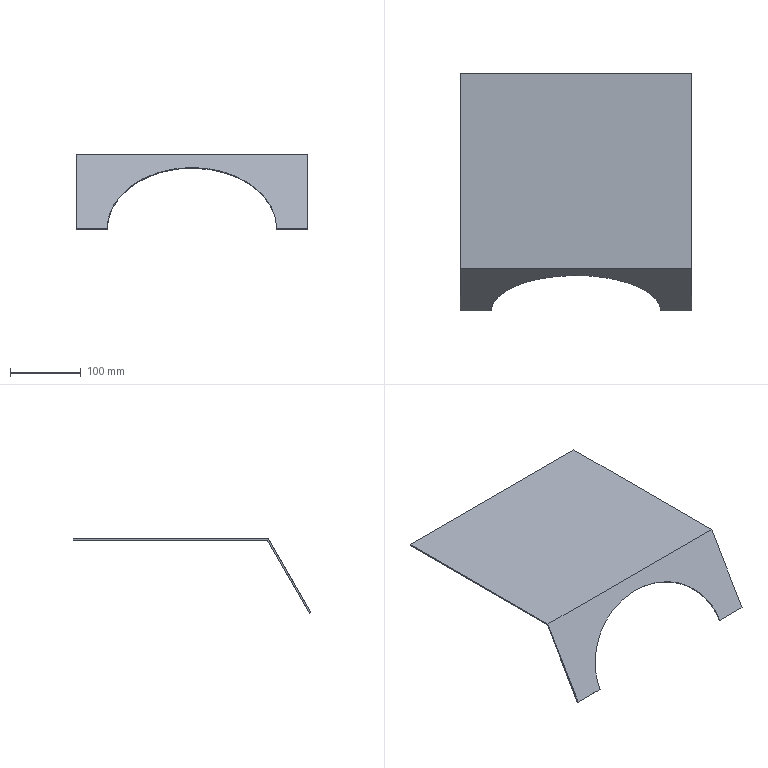Part | SolidWorks | features Attribute 3, ICE 2, Extrusion 1 | 1 solid | 10 faces | box 328 x 336.732 x 105.923 mm | volume 222158 mm3 | plane 9 | spline 1
STEP:
#1=CARTESIAN_POINT('',(-120.,-199.232,-102.923));
#2=VERTEX_POINT('',#1);
#3=CARTESIAN_POINT('',(-120.,-197.5,-103.923));
#4=VERTEX_POINT('',#3);
#5=CARTESIAN_POINT('',(-120.,-206.16,-98.923));
#6=DIRECTION('',(0.,0.866,-0.5));
#7=VECTOR('',#6,1000.);
#8=LINE('',#5,#7);
#9=EDGE_CURVE('',#2,#4,#8,.T.);
#10=ORIENTED_EDGE('',*,*,#9,.F.);
#11=CARTESIAN_POINT('',(-164.,-199.232,-102.923));
#12=VERTEX_POINT('',#11);
#13=CARTESIAN_POINT('',(286.599,-199.232,-102.923));
#14=DIRECTION('',(-1.,0.,0.));
#15=VECTOR('',#14,1000.);
#16=LINE('',#13,#15);
#17=EDGE_CURVE('',#2,#12,#16,.T.);
#18=ORIENTED_EDGE('',*,*,#17,.T.);
#19=CARTESIAN_POINT('',(-164.,-197.5,-103.923));
#20=VERTEX_POINT('',#19);
#21=CARTESIAN_POINT('',(-164.,-197.5,-103.923));
#22=DIRECTION('',(0.,-0.866,0.5));
#23=VECTOR('',#22,1000.);
#24=LINE('',#21,#23);
#25=EDGE_CURVE('',#20,#12,#24,.T.);
#26=ORIENTED_EDGE('',*,*,#25,.F.);
#27=CARTESIAN_POINT('',(286.599,-197.5,-103.923));
#28=DIRECTION('',(-1.,0.,0.));
#29=VECTOR('',#28,1000.);
#30=LINE('',#27,#29);
#31=EDGE_CURVE('',#4,#20,#30,.T.);
#32=ORIENTED_EDGE('',*,*,#31,.F.);
#33=EDGE_LOOP('',(#10,#18,#26,#32));
#34=FACE_OUTER_BOUND('',#33,.T.);
#35=CARTESIAN_POINT('',(286.599,-197.5,-103.923));
#36=DIRECTION('',(0.,-0.5,-0.866));
#37=DIRECTION('',(0.,0.866,-0.5));
#38=AXIS2_PLACEMENT_3D('',#35,#36,#37);
#39=PLANE('',#38);
#40=ADVANCED_FACE('',(#34),#39,.T.);
#41=CARTESIAN_POINT('',(164.,-137.5,0.));
#42=VERTEX_POINT('',#41);
#43=CARTESIAN_POINT('',(164.,137.5,0.));
#44=VERTEX_POINT('',#43);
#45=CARTESIAN_POINT('',(164.,137.5,0.));
#46=DIRECTION('',(0.,1.,0.));
#47=VECTOR('',#46,1000.);
#48=LINE('',#45,#47);
#49=EDGE_CURVE('',#42,#44,#48,.T.);
#50=ORIENTED_EDGE('',*,*,#49,.T.);
#51=CARTESIAN_POINT('',(164.,137.5,2.));
#52=VERTEX_POINT('',#51);
#53=CARTESIAN_POINT('',(164.,137.5,2.));
#54=DIRECTION('',(0.,0.,-1.));
#55=VECTOR('',#54,1000.);
#56=LINE('',#53,#55);
#57=EDGE_CURVE('',#52,#44,#56,.T.);
#58=ORIENTED_EDGE('',*,*,#57,.F.);
#59=CARTESIAN_POINT('',(164.,-138.655,2.));
#60=VERTEX_POINT('',#59);
#61=CARTESIAN_POINT('',(164.,137.5,2.));
#62=DIRECTION('',(0.,1.,0.));
#63=VECTOR('',#62,1000.);
#64=LINE('',#61,#63);
#65=EDGE_CURVE('',#60,#52,#64,.T.);
#66=ORIENTED_EDGE('',*,*,#65,.F.);
#67=CARTESIAN_POINT('',(164.,-199.232,-102.923));
#68=VERTEX_POINT('',#67);
#69=CARTESIAN_POINT('',(164.,-139.232,1.));
#70=DIRECTION('',(0.,-0.5,-0.866));
#71=VECTOR('',#70,1000.);
#72=LINE('',#69,#71);
#73=EDGE_CURVE('',#60,#68,#72,.T.);
#74=ORIENTED_EDGE('',*,*,#73,.T.);
#75=CARTESIAN_POINT('',(164.,-197.5,-103.923));
#76=VERTEX_POINT('',#75);
#77=CARTESIAN_POINT('',(164.,-197.5,-103.923));
#78=DIRECTION('',(0.,0.866,-0.5));
#79=VECTOR('',#78,1000.);
#80=LINE('',#77,#79);
#81=EDGE_CURVE('',#68,#76,#80,.T.);
#82=ORIENTED_EDGE('',*,*,#81,.T.);
#83=CARTESIAN_POINT('',(164.,-137.5,0.));
#84=DIRECTION('',(0.,0.5,0.866));
#85=VECTOR('',#84,1000.);
#86=LINE('',#83,#85);
#87=EDGE_CURVE('',#76,#42,#86,.T.);
#88=ORIENTED_EDGE('',*,*,#87,.T.);
#89=EDGE_LOOP('',(#50,#58,#66,#74,#82,#88));
#90=FACE_OUTER_BOUND('',#89,.T.);
#91=CARTESIAN_POINT('',(164.,137.5,2.));
#92=DIRECTION('',(-1.,0.,0.));
#93=DIRECTION('',(0.,-1.,0.));
#94=AXIS2_PLACEMENT_3D('',#91,#92,#93);
#95=PLANE('',#94);
#96=ADVANCED_FACE('',(#90),#95,.F.);
#97=CARTESIAN_POINT('',(-164.,137.5,0.));
#98=VERTEX_POINT('',#97);
#99=CARTESIAN_POINT('',(-164.,137.5,0.));
#100=DIRECTION('',(-1.,0.,0.));
#101=VECTOR('',#100,1000.);
#102=LINE('',#99,#101);
#103=EDGE_CURVE('',#44,#98,#102,.T.);
#104=ORIENTED_EDGE('',*,*,#103,.T.);
#105=CARTESIAN_POINT('',(-164.,137.5,2.));
#106=VERTEX_POINT('',#105);
#107=CARTESIAN_POINT('',(-164.,137.5,2.));
#108=DIRECTION('',(0.,0.,-1.));
#109=VECTOR('',#108,1000.);
#110=LINE('',#107,#109);
#111=EDGE_CURVE('',#106,#98,#110,.T.);
#112=ORIENTED_EDGE('',*,*,#111,.F.);
#113=CARTESIAN_POINT('',(-164.,137.5,2.));
#114=DIRECTION('',(-1.,0.,0.));
#115=VECTOR('',#114,1000.);
#116=LINE('',#113,#115);
#117=EDGE_CURVE('',#52,#106,#116,.T.);
#118=ORIENTED_EDGE('',*,*,#117,.F.);
#119=ORIENTED_EDGE('',*,*,#57,.T.);
#120=EDGE_LOOP('',(#104,#112,#118,#119));
#121=FACE_OUTER_BOUND('',#120,.T.);
#122=CARTESIAN_POINT('',(-164.,137.5,2.));
#123=DIRECTION('',(0.,-1.,0.));
#124=DIRECTION('',(0.,0.,-1.));
#125=AXIS2_PLACEMENT_3D('',#122,#123,#124);
#126=PLANE('',#125);
#127=ADVANCED_FACE('',(#121),#126,.F.);
#128=CARTESIAN_POINT('',(-164.,-137.5,0.));
#129=VERTEX_POINT('',#128);
#130=CARTESIAN_POINT('',(-164.,137.5,0.));
#131=DIRECTION('',(0.,-1.,0.));
#132=VECTOR('',#131,1000.);
#133=LINE('',#130,#132);
#134=EDGE_CURVE('',#98,#129,#133,.T.);
#135=ORIENTED_EDGE('',*,*,#134,.T.);
#136=CARTESIAN_POINT('',(-164.,-137.5,0.));
#137=DIRECTION('',(0.,-0.5,-0.866));
#138=VECTOR('',#137,1000.);
#139=LINE('',#136,#138);
#140=EDGE_CURVE('',#129,#20,#139,.T.);
#141=ORIENTED_EDGE('',*,*,#140,.T.);
#142=ORIENTED_EDGE('',*,*,#25,.T.);
#143=CARTESIAN_POINT('',(-164.,-138.655,2.));
#144=VERTEX_POINT('',#143);
#145=CARTESIAN_POINT('',(-164.,-139.232,1.));
#146=DIRECTION('',(0.,0.5,0.866));
#147=VECTOR('',#146,1000.);
#148=LINE('',#145,#147);
#149=EDGE_CURVE('',#12,#144,#148,.T.);
#150=ORIENTED_EDGE('',*,*,#149,.T.);
#151=CARTESIAN_POINT('',(-164.,137.5,2.));
#152=DIRECTION('',(0.,-1.,0.));
#153=VECTOR('',#152,1000.);
#154=LINE('',#151,#153);
#155=EDGE_CURVE('',#106,#144,#154,.T.);
#156=ORIENTED_EDGE('',*,*,#155,.F.);
#157=ORIENTED_EDGE('',*,*,#111,.T.);
#158=EDGE_LOOP('',(#135,#141,#142,#150,#156,#157));
#159=FACE_OUTER_BOUND('',#158,.T.);
#160=CARTESIAN_POINT('',(-164.,137.5,2.));
#161=DIRECTION('',(1.,0.,0.));
#162=DIRECTION('',(0.,1.,0.));
#163=AXIS2_PLACEMENT_3D('',#160,#161,#162);
#164=PLANE('',#163);
#165=ADVANCED_FACE('',(#159),#164,.F.);
#166=ORIENTED_EDGE('',*,*,#65,.T.);
#167=ORIENTED_EDGE('',*,*,#117,.T.);
#168=ORIENTED_EDGE('',*,*,#155,.T.);
#169=CARTESIAN_POINT('',(286.599,-138.655,2.));
#170=DIRECTION('',(-1.,0.,0.));
#171=VECTOR('',#170,1000.);
#172=LINE('',#169,#171);
#173=EDGE_CURVE('',#60,#144,#172,.T.);
#174=ORIENTED_EDGE('',*,*,#173,.F.);
#175=EDGE_LOOP('',(#166,#167,#168,#174));
#176=FACE_OUTER_BOUND('',#175,.T.);
#177=CARTESIAN_POINT('',(0.,0.,2.));
#178=DIRECTION('',(0.,0.,1.));
#179=DIRECTION('',(1.,0.,0.));
#180=AXIS2_PLACEMENT_3D('',#177,#178,#179);
#181=PLANE('',#180);
#182=ADVANCED_FACE('',(#176),#181,.T.);
#183=ORIENTED_EDGE('',*,*,#49,.F.);
#184=CARTESIAN_POINT('',(-164.,-137.5,0.));
#185=DIRECTION('',(1.,0.,0.));
#186=VECTOR('',#185,1000.);
#187=LINE('',#184,#186);
#188=EDGE_CURVE('',#129,#42,#187,.T.);
#189=ORIENTED_EDGE('',*,*,#188,.F.);
#190=ORIENTED_EDGE('',*,*,#134,.F.);
#191=ORIENTED_EDGE('',*,*,#103,.F.);
#192=EDGE_LOOP('',(#183,#189,#190,#191));
#193=FACE_OUTER_BOUND('',#192,.T.);
#194=CARTESIAN_POINT('',(0.,0.,0.));
#195=DIRECTION('',(0.,0.,1.));
#196=DIRECTION('',(1.,0.,0.));
#197=AXIS2_PLACEMENT_3D('',#194,#195,#196);
#198=PLANE('',#197);
#199=ADVANCED_FACE('',(#193),#198,.F.);
#200=CARTESIAN_POINT('',(120.,-199.232,-102.923));
#201=VERTEX_POINT('',#200);
#202=CARTESIAN_POINT('',(120.,-199.232,-102.923));
#203=CARTESIAN_POINT('',(120.,-99.232,70.282));
#204=CARTESIAN_POINT('',(-120.,-99.232,70.282));
#205=CARTESIAN_POINT('',(-120.,-199.232,-102.923));
#206=(BOUNDED_CURVE()B_SPLINE_CURVE(3,(#202,#203,#204,#205),.UNSPECIFIED.,.F.,.F.)B_SPLINE_CURVE_WITH_KNOTS((4,4),(0.,3.142),.UNSPECIFIED.)CURVE()GEOMETRIC_REPRESENTATION_ITEM()RATIONAL_B_SPLINE_CURVE((1.,0.3333,0.3333,1.))REPRESENTATION_ITEM(''));
#207=EDGE_CURVE('',#201,#2,#206,.T.);
#208=ORIENTED_EDGE('',*,*,#207,.F.);
#209=CARTESIAN_POINT('',(286.599,-199.232,-102.923));
#210=DIRECTION('',(-1.,0.,0.));
#211=VECTOR('',#210,1000.);
#212=LINE('',#209,#211);
#213=EDGE_CURVE('',#68,#201,#212,.T.);
#214=ORIENTED_EDGE('',*,*,#213,.F.);
#215=ORIENTED_EDGE('',*,*,#73,.F.);
#216=ORIENTED_EDGE('',*,*,#173,.T.);
#217=ORIENTED_EDGE('',*,*,#149,.F.);
#218=ORIENTED_EDGE('',*,*,#17,.F.);
#219=EDGE_LOOP('',(#208,#214,#215,#216,#217,#218));
#220=FACE_OUTER_BOUND('',#219,.T.);
#221=CARTESIAN_POINT('',(286.599,-139.232,1.));
#222=DIRECTION('',(0.,-0.866,0.5));
#223=DIRECTION('',(0.,-0.5,-0.866));
#224=AXIS2_PLACEMENT_3D('',#221,#222,#223);
#225=PLANE('',#224);
#226=ADVANCED_FACE('',(#220),#225,.T.);
#227=CARTESIAN_POINT('',(120.,-197.5,-103.923));
#228=VERTEX_POINT('',#227);
#229=CARTESIAN_POINT('',(120.,-206.16,-98.923));
#230=DIRECTION('',(0.,-0.866,0.5));
#231=VECTOR('',#230,1000.);
#232=LINE('',#229,#231);
#233=EDGE_CURVE('',#228,#201,#232,.T.);
#234=ORIENTED_EDGE('',*,*,#233,.F.);
#235=CARTESIAN_POINT('',(286.599,-197.5,-103.923));
#236=DIRECTION('',(-1.,0.,0.));
#237=VECTOR('',#236,1000.);
#238=LINE('',#235,#237);
#239=EDGE_CURVE('',#76,#228,#238,.T.);
#240=ORIENTED_EDGE('',*,*,#239,.F.);
#241=ORIENTED_EDGE('',*,*,#81,.F.);
#242=ORIENTED_EDGE('',*,*,#213,.T.);
#243=EDGE_LOOP('',(#234,#240,#241,#242));
#244=FACE_OUTER_BOUND('',#243,.T.);
#245=CARTESIAN_POINT('',(286.599,-197.5,-103.923));
#246=DIRECTION('',(0.,-0.5,-0.866));
#247=DIRECTION('',(0.,0.866,-0.5));
#248=AXIS2_PLACEMENT_3D('',#245,#246,#247);
#249=PLANE('',#248);
#250=ADVANCED_FACE('',(#244),#249,.T.);
#251=CARTESIAN_POINT('',(-120.,-197.5,-103.923));
#252=CARTESIAN_POINT('',(-120.,-97.5,69.282));
#253=CARTESIAN_POINT('',(120.,-97.5,69.282));
#254=CARTESIAN_POINT('',(120.,-197.5,-103.923));
#255=(BOUNDED_CURVE()B_SPLINE_CURVE(3,(#251,#252,#253,#254),.UNSPECIFIED.,.F.,.F.)B_SPLINE_CURVE_WITH_KNOTS((4,4),(3.142,6.283),.UNSPECIFIED.)CURVE()GEOMETRIC_REPRESENTATION_ITEM()RATIONAL_B_SPLINE_CURVE((1.,0.3333,0.3333,1.))REPRESENTATION_ITEM(''));
#256=EDGE_CURVE('',#4,#228,#255,.T.);
#257=ORIENTED_EDGE('',*,*,#256,.F.);
#258=ORIENTED_EDGE('',*,*,#31,.T.);
#259=ORIENTED_EDGE('',*,*,#140,.F.);
#260=ORIENTED_EDGE('',*,*,#188,.T.);
#261=ORIENTED_EDGE('',*,*,#87,.F.);
#262=ORIENTED_EDGE('',*,*,#239,.T.);
#263=EDGE_LOOP('',(#257,#258,#259,#260,#261,#262));
#264=FACE_OUTER_BOUND('',#263,.T.);
#265=CARTESIAN_POINT('',(286.599,-137.5,0.));
#266=DIRECTION('',(0.,0.866,-0.5));
#267=DIRECTION('',(0.,0.5,0.866));
#268=AXIS2_PLACEMENT_3D('',#265,#266,#267);
#269=PLANE('',#268);
#270=ADVANCED_FACE('',(#264),#269,.T.);
#271=ORIENTED_EDGE('',*,*,#9,.T.);
#272=ORIENTED_EDGE('',*,*,#256,.T.);
#273=ORIENTED_EDGE('',*,*,#233,.T.);
#274=ORIENTED_EDGE('',*,*,#207,.T.);
#275=EDGE_LOOP('',(#271,#272,#273,#274));
#276=FACE_OUTER_BOUND('',#275,.T.);
#277=CARTESIAN_POINT('',(-120.,-199.232,-102.923));
#278=CARTESIAN_POINT('',(-120.,-197.5,-103.923));
#279=CARTESIAN_POINT('',(-120.,-99.232,70.282));
#280=CARTESIAN_POINT('',(-120.,-97.5,69.282));
#281=CARTESIAN_POINT('',(120.,-99.232,70.282));
#282=CARTESIAN_POINT('',(120.,-97.5,69.282));
#283=CARTESIAN_POINT('',(120.,-199.232,-102.923));
#284=CARTESIAN_POINT('',(120.,-197.5,-103.923));
#285=(BOUNDED_SURFACE()B_SPLINE_SURFACE(3,1,((#277,#278),(#279,#280),(#281,#282),(#283,#284)),.UNSPECIFIED.,.F.,.F.,.F.)B_SPLINE_SURFACE_WITH_KNOTS((4,4),(2,2),(0.,1.),(0.,1.),.UNSPECIFIED.)GEOMETRIC_REPRESENTATION_ITEM()RATIONAL_B_SPLINE_SURFACE(((1.,1.),(0.3333,0.3333),(0.3333,0.3333),(1.,1.)))REPRESENTATION_ITEM('')SURFACE());
#286=ADVANCED_FACE('',(#276),#285,.F.);
#287=CLOSED_SHELL('',(#40,#96,#127,#165,#182,#199,#226,#250,#270,#286));
#288=MANIFOLD_SOLID_BREP('',#287);
#289=CARTESIAN_POINT('',(0.,0.,0.));
#290=DIRECTION('',(0.,0.,1.));
#291=DIRECTION('',(1.,0.,0.));
#292=AXIS2_PLACEMENT_3D('',#289,#290,#291);
#293=(LENGTH_UNIT()NAMED_UNIT(*)SI_UNIT(.MILLI.,.METRE.));
#294=UNCERTAINTY_MEASURE_WITH_UNIT(LENGTH_MEASURE(0.00001),#293,'','');
#295=(NAMED_UNIT(*)PLANE_ANGLE_UNIT()SI_UNIT($,.RADIAN.));
#296=(NAMED_UNIT(*)SI_UNIT($,.STERADIAN.)SOLID_ANGLE_UNIT());
#297=(GEOMETRIC_REPRESENTATION_CONTEXT(3)GLOBAL_UNCERTAINTY_ASSIGNED_CONTEXT((#294))GLOBAL_UNIT_ASSIGNED_CONTEXT((#293,#295,#296))REPRESENTATION_CONTEXT('',''));
#298=ADVANCED_BREP_SHAPE_REPRESENTATION('',(#288,#292),#297);